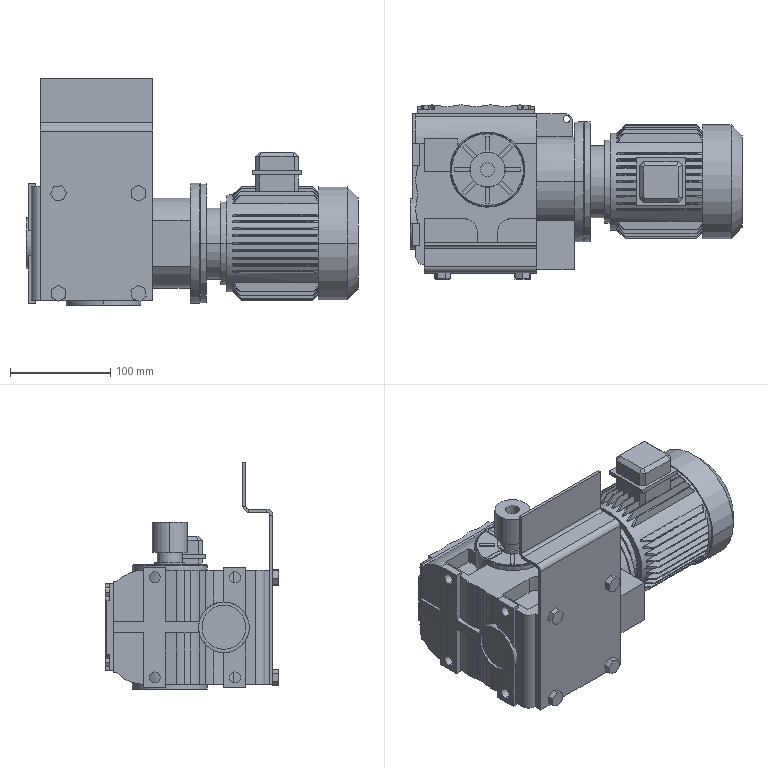Part | STEP file | Produce dryer conveyor belt NSNS47 reducer_NS 67 | 3 solids | 613 faces | box 331.6 x 173.674 x 227.5 mm | volume 3816631 mm3 | plane 435 | cylinder 92 | cone 86 | commonest cylinder face diameters 11 x24 55 x13 30 x6 22 x4 71.8 x4 75 x4